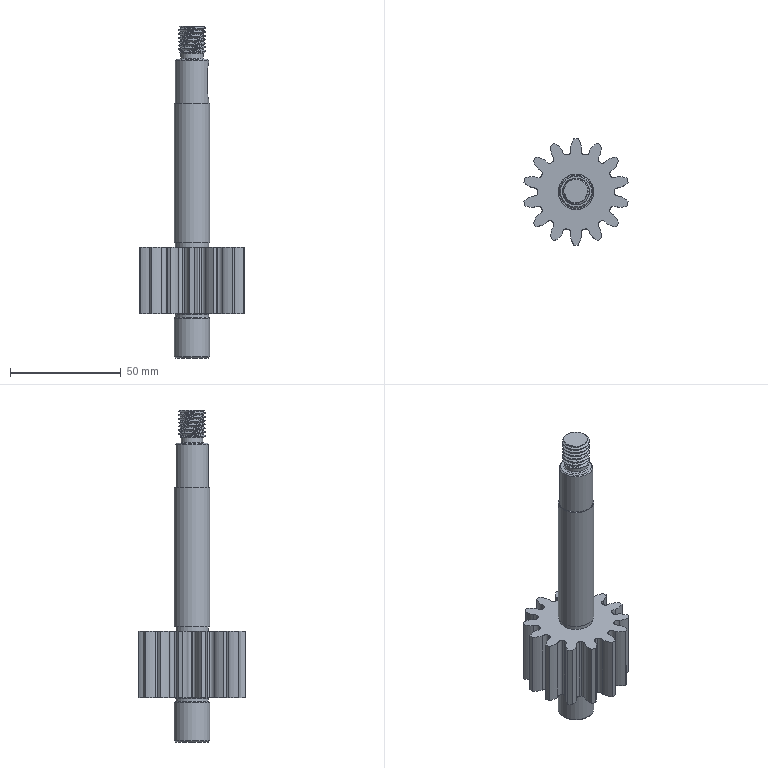Part | NX | features BREP 14, META 14, CYLINDER 5, DATUM_CSYS 5, DATUM_PLANE 4, EXTRUDE 4, SKETCH 4, CHAMFER 3, BLEND 1, FSET 1, THREADS 1 | 1 solid | 116 faces | box 47.19 x 48 x 150 mm | volume 62108 mm3 | spline 72 | cylinder 24 | plane 13 | torus 4 | cone 3 | commonest cylinder face diameters 34.5 x14 15 x3 5 x2 16 x2 10 x1 10.25 x1